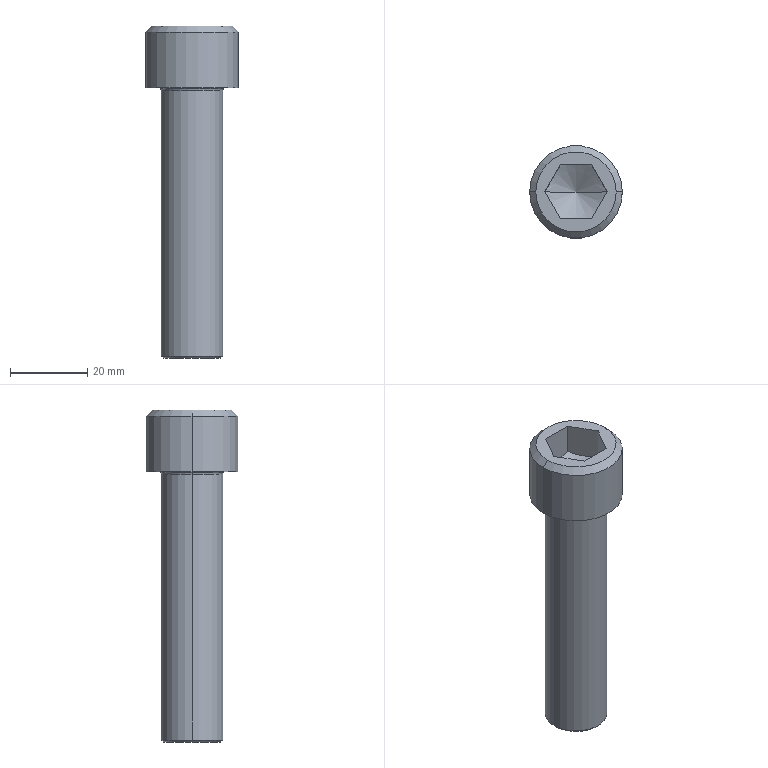Part | Creo | 1 solid | 23 faces | box 24 x 24 x 86 mm | volume 19550 mm3 | plane 9 | cone 6 | cylinder 4 | torus 4 | commonest cylinder face diameters 16 x2 24 x2
STEP:
#1=CARTESIAN_POINT('',(253.083,119.995,322.56));
#2=VERTEX_POINT('',#1);
#3=CARTESIAN_POINT('',(249.041,126.995,322.56));
#4=VERTEX_POINT('',#3);
#5=CARTESIAN_POINT('',(253.083,119.995,322.56));
#6=CARTESIAN_POINT('',(252.894,120.322,322.451));
#7=CARTESIAN_POINT('',(252.516,120.977,322.255));
#8=CARTESIAN_POINT('',(251.94,121.975,322.043));
#9=CARTESIAN_POINT('',(251.358,122.984,321.93));
#10=CARTESIAN_POINT('',(250.769,124.003,321.93));
#11=CARTESIAN_POINT('',(250.186,125.014,322.043));
#12=CARTESIAN_POINT('',(249.61,126.01,322.254));
#13=CARTESIAN_POINT('',(249.231,126.667,322.451));
#14=CARTESIAN_POINT('',(249.041,126.995,322.56));
#15=B_SPLINE_CURVE_WITH_KNOTS('',3,(#5,#6,#7,#8,#9,#10,#11,#12,#13,#14),.UNSPECIFIED.,.F.,.F.,(4,1,1,1,1,1,1,4),(0.,0.1429,0.2857,0.4286,0.5714,0.7143,0.8571,1.),.UNSPECIFIED.);
#16=EDGE_CURVE('',#2,#4,#15,.T.);
#17=ORIENTED_EDGE('',*,*,#16,.F.);
#18=CARTESIAN_POINT('',(245.,119.995,317.893));
#19=VERTEX_POINT('',#18);
#20=CARTESIAN_POINT('',(245.,119.995,317.893));
#21=DIRECTION('',(0.866,0.,0.5));
#22=VECTOR('',#21,9.333);
#23=LINE('',#20,#22);
#24=EDGE_CURVE('',#19,#2,#23,.T.);
#25=ORIENTED_EDGE('',*,*,#24,.F.);
#26=CARTESIAN_POINT('',(236.917,119.995,322.56));
#27=VERTEX_POINT('',#26);
#28=CARTESIAN_POINT('',(245.,119.995,317.893));
#29=DIRECTION('',(-0.866,0.,0.5));
#30=VECTOR('',#29,9.333);
#31=LINE('',#28,#30);
#32=EDGE_CURVE('',#19,#27,#31,.T.);
#33=ORIENTED_EDGE('',*,*,#32,.T.);
#34=CARTESIAN_POINT('',(240.959,126.995,322.56));
#35=VERTEX_POINT('',#34);
#36=CARTESIAN_POINT('',(240.959,126.995,322.56));
#37=CARTESIAN_POINT('',(240.77,126.669,322.451));
#38=CARTESIAN_POINT('',(240.391,126.013,322.255));
#39=CARTESIAN_POINT('',(239.816,125.016,322.043));
#40=CARTESIAN_POINT('',(239.233,124.007,321.93));
#41=CARTESIAN_POINT('',(238.644,122.987,321.93));
#42=CARTESIAN_POINT('',(238.061,121.977,322.043));
#43=CARTESIAN_POINT('',(237.486,120.981,322.254));
#44=CARTESIAN_POINT('',(237.106,120.323,322.451));
#45=CARTESIAN_POINT('',(236.917,119.995,322.56));
#46=B_SPLINE_CURVE_WITH_KNOTS('',3,(#36,#37,#38,#39,#40,#41,#42,#43,#44,#45),.UNSPECIFIED.,.F.,.F.,(4,1,1,1,1,1,1,4),(0.,0.1429,0.2857,0.4286,0.5714,0.7143,0.8571,1.),.UNSPECIFIED.);
#47=EDGE_CURVE('',#35,#27,#46,.T.);
#48=ORIENTED_EDGE('',*,*,#47,.F.);
#49=CARTESIAN_POINT('',(249.041,126.995,322.56));
#50=CARTESIAN_POINT('',(248.667,126.995,322.452));
#51=CARTESIAN_POINT('',(247.914,126.995,322.257));
#52=CARTESIAN_POINT('',(246.756,126.995,322.043));
#53=CARTESIAN_POINT('',(245.587,126.995,321.93));
#54=CARTESIAN_POINT('',(244.417,126.995,321.93));
#55=CARTESIAN_POINT('',(243.25,126.995,322.042));
#56=CARTESIAN_POINT('',(242.092,126.995,322.255));
#57=CARTESIAN_POINT('',(241.335,126.995,322.451));
#58=CARTESIAN_POINT('',(240.959,126.995,322.56));
#59=B_SPLINE_CURVE_WITH_KNOTS('',3,(#49,#50,#51,#52,#53,#54,#55,#56,#57,#58),.UNSPECIFIED.,.F.,.F.,(4,1,1,1,1,1,1,4),(0.,0.1429,0.2857,0.4286,0.5714,0.7143,0.8571,1.),.UNSPECIFIED.);
#60=EDGE_CURVE('',#4,#35,#59,.T.);
#61=ORIENTED_EDGE('',*,*,#60,.F.);
#62=EDGE_LOOP('',(#17,#25,#33,#48,#61));
#63=FACE_OUTER_BOUND('',#62,.F.);
#64=CARTESIAN_POINT('',(245.,119.995,320.273));
#65=DIRECTION('',(0.,0.,1.));
#66=DIRECTION('',(1.,0.,0.));
#67=AXIS2_PLACEMENT_3D('',#64,#65,#66);
#68=CONICAL_SURFACE('',#67,4.122,60.);
#69=ADVANCED_FACE('',(#63),#68,.F.);
#70=CARTESIAN_POINT('',(249.041,126.995,330.56));
#71=VERTEX_POINT('',#70);
#72=CARTESIAN_POINT('',(253.083,119.995,330.56));
#73=VERTEX_POINT('',#72);
#74=CARTESIAN_POINT('',(249.041,126.995,330.56));
#75=DIRECTION('',(0.5,-0.866,0.));
#76=VECTOR('',#75,8.083);
#77=LINE('',#74,#76);
#78=EDGE_CURVE('',#71,#73,#77,.T.);
#79=ORIENTED_EDGE('',*,*,#78,.T.);
#80=CARTESIAN_POINT('',(253.083,119.995,330.56));
#81=DIRECTION('',(0.,0.,-1.));
#82=VECTOR('',#81,8.);
#83=LINE('',#80,#82);
#84=EDGE_CURVE('',#73,#2,#83,.T.);
#85=ORIENTED_EDGE('',*,*,#84,.T.);
#86=ORIENTED_EDGE('',*,*,#16,.T.);
#87=CARTESIAN_POINT('',(249.041,126.995,330.56));
#88=DIRECTION('',(0.,0.,-1.));
#89=VECTOR('',#88,8.);
#90=LINE('',#87,#89);
#91=EDGE_CURVE('',#71,#4,#90,.T.);
#92=ORIENTED_EDGE('',*,*,#91,.F.);
#93=EDGE_LOOP('',(#79,#85,#86,#92));
#94=FACE_OUTER_BOUND('',#93,.F.);
#95=CARTESIAN_POINT('',(249.041,126.995,322.56));
#96=DIRECTION('',(-0.866,-0.5,0.));
#97=DIRECTION('',(0.5,-0.866,0.));
#98=AXIS2_PLACEMENT_3D('',#95,#96,#97);
#99=PLANE('',#98);
#100=ADVANCED_FACE('',(#94),#99,.T.);
#101=CARTESIAN_POINT('',(255.4,119.995,330.56));
#102=VERTEX_POINT('',#101);
#103=CARTESIAN_POINT('',(234.6,119.995,330.56));
#104=VERTEX_POINT('',#103);
#105=CARTESIAN_POINT('',(245.,119.995,330.56));
#106=DIRECTION('',(0.,0.,1.));
#107=DIRECTION('',(1.,0.,0.));
#108=AXIS2_PLACEMENT_3D('',#105,#106,#107);
#109=CIRCLE('',#108,10.4);
#110=EDGE_CURVE('',#102,#104,#109,.T.);
#111=ORIENTED_EDGE('',*,*,#110,.F.);
#112=CARTESIAN_POINT('',(245.,119.995,330.56));
#113=DIRECTION('',(0.,0.,1.));
#114=DIRECTION('',(-1.,0.,0.));
#115=AXIS2_PLACEMENT_3D('',#112,#113,#114);
#116=CIRCLE('',#115,10.4);
#117=EDGE_CURVE('',#104,#102,#116,.T.);
#118=ORIENTED_EDGE('',*,*,#117,.F.);
#119=EDGE_LOOP('',(#111,#118));
#120=FACE_OUTER_BOUND('',#119,.F.);
#121=CARTESIAN_POINT('',(249.041,112.995,330.56));
#122=VERTEX_POINT('',#121);
#123=CARTESIAN_POINT('',(253.083,119.995,330.56));
#124=DIRECTION('',(-0.5,-0.866,0.));
#125=VECTOR('',#124,8.083);
#126=LINE('',#123,#125);
#127=EDGE_CURVE('',#73,#122,#126,.T.);
#128=ORIENTED_EDGE('',*,*,#127,.F.);
#129=ORIENTED_EDGE('',*,*,#78,.F.);
#130=CARTESIAN_POINT('',(240.959,126.995,330.56));
#131=VERTEX_POINT('',#130);
#132=CARTESIAN_POINT('',(249.041,126.995,330.56));
#133=DIRECTION('',(-1.,0.,0.));
#134=VECTOR('',#133,8.083);
#135=LINE('',#132,#134);
#136=EDGE_CURVE('',#71,#131,#135,.T.);
#137=ORIENTED_EDGE('',*,*,#136,.T.);
#138=CARTESIAN_POINT('',(236.917,119.995,330.56));
#139=VERTEX_POINT('',#138);
#140=CARTESIAN_POINT('',(236.917,119.995,330.56));
#141=DIRECTION('',(0.5,0.866,0.));
#142=VECTOR('',#141,8.083);
#143=LINE('',#140,#142);
#144=EDGE_CURVE('',#139,#131,#143,.T.);
#145=ORIENTED_EDGE('',*,*,#144,.F.);
#146=CARTESIAN_POINT('',(240.959,112.995,330.56));
#147=VERTEX_POINT('',#146);
#148=CARTESIAN_POINT('',(240.959,112.995,330.56));
#149=DIRECTION('',(-0.5,0.866,0.));
#150=VECTOR('',#149,8.083);
#151=LINE('',#148,#150);
#152=EDGE_CURVE('',#147,#139,#151,.T.);
#153=ORIENTED_EDGE('',*,*,#152,.F.);
#154=CARTESIAN_POINT('',(240.959,112.995,330.56));
#155=DIRECTION('',(1.,0.,0.));
#156=VECTOR('',#155,8.083);
#157=LINE('',#154,#156);
#158=EDGE_CURVE('',#147,#122,#157,.T.);
#159=ORIENTED_EDGE('',*,*,#158,.T.);
#160=EDGE_LOOP('',(#128,#129,#137,#145,#153,#159));
#161=FACE_BOUND('',#160,.F.);
#162=CARTESIAN_POINT('',(245.,119.995,330.56));
#163=DIRECTION('',(0.,0.,1.));
#164=DIRECTION('',(1.,0.,0.));
#165=AXIS2_PLACEMENT_3D('',#162,#163,#164);
#166=PLANE('',#165);
#167=ADVANCED_FACE('',(#120,#161),#166,.T.);
#168=CARTESIAN_POINT('',(257.,119.995,328.96));
#169=VERTEX_POINT('',#168);
#170=CARTESIAN_POINT('',(233.,119.995,328.96));
#171=VERTEX_POINT('',#170);
#172=CARTESIAN_POINT('',(245.,119.995,328.96));
#173=DIRECTION('',(0.,0.,1.));
#174=DIRECTION('',(1.,0.,0.));
#175=AXIS2_PLACEMENT_3D('',#172,#173,#174);
#176=CIRCLE('',#175,12.);
#177=EDGE_CURVE('',#169,#171,#176,.T.);
#178=ORIENTED_EDGE('',*,*,#177,.F.);
#179=CARTESIAN_POINT('',(255.4,119.995,330.56));
#180=DIRECTION('',(0.7071,0.,-0.7071));
#181=VECTOR('',#180,2.263);
#182=LINE('',#179,#181);
#183=EDGE_CURVE('',#102,#169,#182,.T.);
#184=ORIENTED_EDGE('',*,*,#183,.F.);
#185=ORIENTED_EDGE('',*,*,#110,.T.);
#186=CARTESIAN_POINT('',(234.6,119.995,330.56));
#187=DIRECTION('',(-0.7071,0.,-0.7071));
#188=VECTOR('',#187,2.263);
#189=LINE('',#186,#188);
#190=EDGE_CURVE('',#104,#171,#189,.T.);
#191=ORIENTED_EDGE('',*,*,#190,.T.);
#192=EDGE_LOOP('',(#178,#184,#185,#191));
#193=FACE_OUTER_BOUND('',#192,.F.);
#194=CARTESIAN_POINT('',(245.,119.995,329.76));
#195=DIRECTION('',(0.,0.,-1.));
#196=DIRECTION('',(-1.,0.,0.));
#197=AXIS2_PLACEMENT_3D('',#194,#195,#196);
#198=CONICAL_SURFACE('',#197,11.2,45.);
#199=ADVANCED_FACE('',(#193),#198,.T.);
#200=ORIENTED_EDGE('',*,*,#177,.T.);
#201=CARTESIAN_POINT('',(233.,119.995,314.56));
#202=VERTEX_POINT('',#201);
#203=CARTESIAN_POINT('',(233.,119.995,314.56));
#204=DIRECTION('',(0.,0.,1.));
#205=VECTOR('',#204,14.4);
#206=LINE('',#203,#205);
#207=EDGE_CURVE('',#202,#171,#206,.T.);
#208=ORIENTED_EDGE('',*,*,#207,.F.);
#209=CARTESIAN_POINT('',(257.,119.995,314.56));
#210=VERTEX_POINT('',#209);
#211=CARTESIAN_POINT('',(245.,119.995,314.56));
#212=DIRECTION('',(0.,0.,-1.));
#213=DIRECTION('',(-1.,0.,0.));
#214=AXIS2_PLACEMENT_3D('',#211,#212,#213);
#215=CIRCLE('',#214,12.);
#216=EDGE_CURVE('',#202,#210,#215,.T.);
#217=ORIENTED_EDGE('',*,*,#216,.T.);
#218=CARTESIAN_POINT('',(257.,119.995,314.56));
#219=DIRECTION('',(0.,0.,1.));
#220=VECTOR('',#219,14.4);
#221=LINE('',#218,#220);
#222=EDGE_CURVE('',#210,#169,#221,.T.);
#223=ORIENTED_EDGE('',*,*,#222,.T.);
#224=EDGE_LOOP('',(#200,#208,#217,#223));
#225=FACE_OUTER_BOUND('',#224,.F.);
#226=CARTESIAN_POINT('',(245.,119.995,314.56));
#227=DIRECTION('',(0.,0.,1.));
#228=DIRECTION('',(1.,0.,0.));
#229=AXIS2_PLACEMENT_3D('',#226,#227,#228);
#230=CYLINDRICAL_SURFACE('',#229,12.);
#231=ADVANCED_FACE('',(#225),#230,.T.);
#232=CARTESIAN_POINT('',(245.,119.995,328.96));
#233=DIRECTION('',(0.,0.,1.));
#234=DIRECTION('',(-1.,0.,0.));
#235=AXIS2_PLACEMENT_3D('',#232,#233,#234);
#236=CIRCLE('',#235,12.);
#237=EDGE_CURVE('',#171,#169,#236,.T.);
#238=ORIENTED_EDGE('',*,*,#237,.T.);
#239=ORIENTED_EDGE('',*,*,#222,.F.);
#240=CARTESIAN_POINT('',(245.,119.995,314.56));
#241=DIRECTION('',(0.,0.,-1.));
#242=DIRECTION('',(1.,0.,0.));
#243=AXIS2_PLACEMENT_3D('',#240,#241,#242);
#244=CIRCLE('',#243,12.);
#245=EDGE_CURVE('',#210,#202,#244,.T.);
#246=ORIENTED_EDGE('',*,*,#245,.T.);
#247=ORIENTED_EDGE('',*,*,#207,.T.);
#248=EDGE_LOOP('',(#238,#239,#246,#247));
#249=FACE_OUTER_BOUND('',#248,.F.);
#250=CARTESIAN_POINT('',(245.,119.995,314.56));
#251=DIRECTION('',(0.,0.,1.));
#252=DIRECTION('',(1.,0.,0.));
#253=AXIS2_PLACEMENT_3D('',#250,#251,#252);
#254=CYLINDRICAL_SURFACE('',#253,12.);
#255=ADVANCED_FACE('',(#249),#254,.T.);
#256=ORIENTED_EDGE('',*,*,#237,.F.);
#257=ORIENTED_EDGE('',*,*,#190,.F.);
#258=ORIENTED_EDGE('',*,*,#117,.T.);
#259=ORIENTED_EDGE('',*,*,#183,.T.);
#260=EDGE_LOOP('',(#256,#257,#258,#259));
#261=FACE_OUTER_BOUND('',#260,.F.);
#262=CARTESIAN_POINT('',(245.,119.995,329.76));
#263=DIRECTION('',(0.,0.,-1.));
#264=DIRECTION('',(-1.,0.,0.));
#265=AXIS2_PLACEMENT_3D('',#262,#263,#264);
#266=CONICAL_SURFACE('',#265,11.2,45.);
#267=ADVANCED_FACE('',(#261),#266,.T.);
#268=ORIENTED_EDGE('',*,*,#245,.F.);
#269=ORIENTED_EDGE('',*,*,#216,.F.);
#270=EDGE_LOOP('',(#268,#269));
#271=FACE_OUTER_BOUND('',#270,.F.);
#272=CARTESIAN_POINT('',(253.6,119.995,314.56));
#273=VERTEX_POINT('',#272);
#274=CARTESIAN_POINT('',(236.4,119.995,314.56));
#275=VERTEX_POINT('',#274);
#276=CARTESIAN_POINT('',(245.,119.995,314.56));
#277=DIRECTION('',(0.,0.,1.));
#278=DIRECTION('',(1.,0.,0.));
#279=AXIS2_PLACEMENT_3D('',#276,#277,#278);
#280=CIRCLE('',#279,8.6);
#281=EDGE_CURVE('',#273,#275,#280,.T.);
#282=ORIENTED_EDGE('',*,*,#281,.F.);
#283=CARTESIAN_POINT('',(245.,119.995,314.56));
#284=DIRECTION('',(0.,0.,1.));
#285=DIRECTION('',(-1.,0.,0.));
#286=AXIS2_PLACEMENT_3D('',#283,#284,#285);
#287=CIRCLE('',#286,8.6);
#288=EDGE_CURVE('',#275,#273,#287,.T.);
#289=ORIENTED_EDGE('',*,*,#288,.F.);
#290=EDGE_LOOP('',(#282,#289));
#291=FACE_BOUND('',#290,.F.);
#292=CARTESIAN_POINT('',(245.,119.995,314.56));
#293=DIRECTION('',(0.,0.,1.));
#294=DIRECTION('',(1.,0.,0.));
#295=AXIS2_PLACEMENT_3D('',#292,#293,#294);
#296=PLANE('',#295);
#297=ADVANCED_FACE('',(#271,#291),#296,.F.);
#298=ORIENTED_EDGE('',*,*,#281,.T.);
#299=CARTESIAN_POINT('',(236.824,119.995,314.384));
#300=VERTEX_POINT('',#299);
#301=CARTESIAN_POINT('',(236.4,119.995,313.96));
#302=DIRECTION('',(0.,1.,0.));
#303=DIRECTION('',(0.,0.,1.));
#304=AXIS2_PLACEMENT_3D('',#301,#302,#303);
#305=CIRCLE('',#304,0.6);
#306=EDGE_CURVE('',#275,#300,#305,.T.);
#307=ORIENTED_EDGE('',*,*,#306,.T.);
#308=CARTESIAN_POINT('',(253.176,119.995,314.384));
#309=VERTEX_POINT('',#308);
#310=CARTESIAN_POINT('',(245.,119.995,314.384));
#311=DIRECTION('',(0.,0.,1.));
#312=DIRECTION('',(1.,0.,0.));
#313=AXIS2_PLACEMENT_3D('',#310,#311,#312);
#314=CIRCLE('',#313,8.176);
#315=EDGE_CURVE('',#309,#300,#314,.T.);
#316=ORIENTED_EDGE('',*,*,#315,.F.);
#317=CARTESIAN_POINT('',(253.6,119.995,313.96));
#318=DIRECTION('',(0.,-1.,0.));
#319=DIRECTION('',(0.,0.,1.));
#320=AXIS2_PLACEMENT_3D('',#317,#318,#319);
#321=CIRCLE('',#320,0.6);
#322=EDGE_CURVE('',#273,#309,#321,.T.);
#323=ORIENTED_EDGE('',*,*,#322,.F.);
#324=EDGE_LOOP('',(#298,#307,#316,#323));
#325=FACE_OUTER_BOUND('',#324,.F.);
#326=CARTESIAN_POINT('',(245.,119.995,313.96));
#327=DIRECTION('',(0.,0.,1.));
#328=DIRECTION('',(1.,0.,0.));
#329=AXIS2_PLACEMENT_3D('',#326,#327,#328);
#330=TOROIDAL_SURFACE('',#329,8.6,0.6);
#331=ADVANCED_FACE('',(#325),#330,.F.);
#332=ORIENTED_EDGE('',*,*,#288,.T.);
#333=ORIENTED_EDGE('',*,*,#322,.T.);
#334=CARTESIAN_POINT('',(245.,119.995,314.384));
#335=DIRECTION('',(0.,0.,1.));
#336=DIRECTION('',(-1.,0.,0.));
#337=AXIS2_PLACEMENT_3D('',#334,#335,#336);
#338=CIRCLE('',#337,8.176);
#339=EDGE_CURVE('',#300,#309,#338,.T.);
#340=ORIENTED_EDGE('',*,*,#339,.F.);
#341=ORIENTED_EDGE('',*,*,#306,.F.);
#342=EDGE_LOOP('',(#332,#333,#340,#341));
#343=FACE_OUTER_BOUND('',#342,.F.);
#344=CARTESIAN_POINT('',(245.,119.995,313.96));
#345=DIRECTION('',(0.,0.,1.));
#346=DIRECTION('',(1.,0.,0.));
#347=AXIS2_PLACEMENT_3D('',#344,#345,#346);
#348=TOROIDAL_SURFACE('',#347,8.6,0.6);
#349=ADVANCED_FACE('',(#343),#348,.F.);
#350=CARTESIAN_POINT('',(237.,119.995,313.96));
#351=VERTEX_POINT('',#350);
#352=CARTESIAN_POINT('',(253.,119.995,313.96));
#353=VERTEX_POINT('',#352);
#354=CARTESIAN_POINT('',(245.,119.995,313.96));
#355=DIRECTION('',(0.,0.,1.));
#356=DIRECTION('',(-1.,0.,0.));
#357=AXIS2_PLACEMENT_3D('',#354,#355,#356);
#358=CIRCLE('',#357,8.);
#359=EDGE_CURVE('',#351,#353,#358,.T.);
#360=ORIENTED_EDGE('',*,*,#359,.F.);
#361=CARTESIAN_POINT('',(236.4,119.995,313.96));
#362=DIRECTION('',(0.,1.,0.));
#363=DIRECTION('',(0.7071,0.,0.7071));
#364=AXIS2_PLACEMENT_3D('',#361,#362,#363);
#365=CIRCLE('',#364,0.6);
#366=EDGE_CURVE('',#300,#351,#365,.T.);
#367=ORIENTED_EDGE('',*,*,#366,.F.);
#368=ORIENTED_EDGE('',*,*,#339,.T.);
#369=CARTESIAN_POINT('',(253.6,119.995,313.96));
#370=DIRECTION('',(0.,-1.,0.));
#371=DIRECTION('',(-0.7071,0.,0.7071));
#372=AXIS2_PLACEMENT_3D('',#369,#370,#371);
#373=CIRCLE('',#372,0.6);
#374=EDGE_CURVE('',#309,#353,#373,.T.);
#375=ORIENTED_EDGE('',*,*,#374,.T.);
#376=EDGE_LOOP('',(#360,#367,#368,#375));
#377=FACE_OUTER_BOUND('',#376,.F.);
#378=CARTESIAN_POINT('',(245.,119.995,313.96));
#379=DIRECTION('',(0.,0.,1.));
#380=DIRECTION('',(1.,0.,0.));
#381=AXIS2_PLACEMENT_3D('',#378,#379,#380);
#382=TOROIDAL_SURFACE('',#381,8.6,0.6);
#383=ADVANCED_FACE('',(#377),#382,.F.);
#384=CARTESIAN_POINT('',(253.,119.995,245.06));
#385=VERTEX_POINT('',#384);
#386=CARTESIAN_POINT('',(237.,119.995,245.06));
#387=VERTEX_POINT('',#386);
#388=CARTESIAN_POINT('',(245.,119.995,245.06));
#389=DIRECTION('',(0.,0.,-1.));
#390=DIRECTION('',(1.,0.,0.));
#391=AXIS2_PLACEMENT_3D('',#388,#389,#390);
#392=CIRCLE('',#391,8.);
#393=EDGE_CURVE('',#385,#387,#392,.T.);
#394=ORIENTED_EDGE('',*,*,#393,.T.);
#395=CARTESIAN_POINT('',(237.,119.995,245.06));
#396=DIRECTION('',(0.,0.,1.));
#397=VECTOR('',#396,68.9);
#398=LINE('',#395,#397);
#399=EDGE_CURVE('',#387,#351,#398,.T.);
#400=ORIENTED_EDGE('',*,*,#399,.T.);
#401=ORIENTED_EDGE('',*,*,#359,.T.);
#402=CARTESIAN_POINT('',(253.,119.995,245.06));
#403=DIRECTION('',(0.,0.,1.));
#404=VECTOR('',#403,68.9);
#405=LINE('',#402,#404);
#406=EDGE_CURVE('',#385,#353,#405,.T.);
#407=ORIENTED_EDGE('',*,*,#406,.F.);
#408=EDGE_LOOP('',(#394,#400,#401,#407));
#409=FACE_OUTER_BOUND('',#408,.F.);
#410=CARTESIAN_POINT('',(245.,119.995,244.56));
#411=DIRECTION('',(0.,0.,1.));
#412=DIRECTION('',(1.,0.,0.));
#413=AXIS2_PLACEMENT_3D('',#410,#411,#412);
#414=CYLINDRICAL_SURFACE('',#413,8.);
#415=ADVANCED_FACE('',(#409),#414,.T.);
#416=CARTESIAN_POINT('',(252.5,119.995,244.56));
#417=VERTEX_POINT('',#416);
#418=CARTESIAN_POINT('',(237.5,119.995,244.56));
#419=VERTEX_POINT('',#418);
#420=CARTESIAN_POINT('',(245.,119.995,244.56));
#421=DIRECTION('',(0.,0.,-1.));
#422=DIRECTION('',(1.,0.,0.));
#423=AXIS2_PLACEMENT_3D('',#420,#421,#422);
#424=CIRCLE('',#423,7.5);
#425=EDGE_CURVE('',#417,#419,#424,.T.);
#426=ORIENTED_EDGE('',*,*,#425,.T.);
#427=CARTESIAN_POINT('',(237.5,119.995,244.56));
#428=DIRECTION('',(-0.7071,0.,0.7071));
#429=VECTOR('',#428,0.7071);
#430=LINE('',#427,#429);
#431=EDGE_CURVE('',#419,#387,#430,.T.);
#432=ORIENTED_EDGE('',*,*,#431,.T.);
#433=ORIENTED_EDGE('',*,*,#393,.F.);
#434=CARTESIAN_POINT('',(252.5,119.995,244.56));
#435=DIRECTION('',(0.7071,0.,0.7071));
#436=VECTOR('',#435,0.7071);
#437=LINE('',#434,#436);
#438=EDGE_CURVE('',#417,#385,#437,.T.);
#439=ORIENTED_EDGE('',*,*,#438,.F.);
#440=EDGE_LOOP('',(#426,#432,#433,#439));
#441=FACE_OUTER_BOUND('',#440,.F.);
#442=CARTESIAN_POINT('',(245.,119.995,244.81));
#443=DIRECTION('',(0.,0.,1.));
#444=DIRECTION('',(1.,0.,0.));
#445=AXIS2_PLACEMENT_3D('',#442,#443,#444);
#446=CONICAL_SURFACE('',#445,7.75,45.);
#447=ADVANCED_FACE('',(#441),#446,.T.);
#448=ORIENTED_EDGE('',*,*,#425,.F.);
#449=CARTESIAN_POINT('',(245.,119.995,244.56));
#450=DIRECTION('',(0.,0.,-1.));
#451=DIRECTION('',(-1.,0.,0.));
#452=AXIS2_PLACEMENT_3D('',#449,#450,#451);
#453=CIRCLE('',#452,7.5);
#454=EDGE_CURVE('',#419,#417,#453,.T.);
#455=ORIENTED_EDGE('',*,*,#454,.F.);
#456=EDGE_LOOP('',(#448,#455));
#457=FACE_OUTER_BOUND('',#456,.F.);
#458=CARTESIAN_POINT('',(245.,119.995,244.56));
#459=DIRECTION('',(0.,0.,1.));
#460=DIRECTION('',(1.,0.,0.));
#461=AXIS2_PLACEMENT_3D('',#458,#459,#460);
#462=PLANE('',#461);
#463=ADVANCED_FACE('',(#457),#462,.F.);
#464=ORIENTED_EDGE('',*,*,#454,.T.);
#465=ORIENTED_EDGE('',*,*,#438,.T.);
#466=CARTESIAN_POINT('',(245.,119.995,245.06));
#467=DIRECTION('',(0.,0.,-1.));
#468=DIRECTION('',(-1.,0.,0.));
#469=AXIS2_PLACEMENT_3D('',#466,#467,#468);
#470=CIRCLE('',#469,8.);
#471=EDGE_CURVE('',#387,#385,#470,.T.);
#472=ORIENTED_EDGE('',*,*,#471,.F.);
#473=ORIENTED_EDGE('',*,*,#431,.F.);
#474=EDGE_LOOP('',(#464,#465,#472,#473));
#475=FACE_OUTER_BOUND('',#474,.F.);
#476=CARTESIAN_POINT('',(245.,119.995,244.81));
#477=DIRECTION('',(0.,0.,1.));
#478=DIRECTION('',(1.,0.,0.));
#479=AXIS2_PLACEMENT_3D('',#476,#477,#478);
#480=CONICAL_SURFACE('',#479,7.75,45.);
#481=ADVANCED_FACE('',(#475),#480,.T.);
#482=ORIENTED_EDGE('',*,*,#471,.T.);
#483=ORIENTED_EDGE('',*,*,#406,.T.);
#484=CARTESIAN_POINT('',(245.,119.995,313.96));
#485=DIRECTION('',(0.,0.,1.));
#486=DIRECTION('',(1.,0.,0.));
#487=AXIS2_PLACEMENT_3D('',#484,#485,#486);
#488=CIRCLE('',#487,8.);
#489=EDGE_CURVE('',#353,#351,#488,.T.);
#490=ORIENTED_EDGE('',*,*,#489,.T.);
#491=ORIENTED_EDGE('',*,*,#399,.F.);
#492=EDGE_LOOP('',(#482,#483,#490,#491));
#493=FACE_OUTER_BOUND('',#492,.F.);
#494=CARTESIAN_POINT('',(245.,119.995,244.56));
#495=DIRECTION('',(0.,0.,1.));
#496=DIRECTION('',(1.,0.,0.));
#497=AXIS2_PLACEMENT_3D('',#494,#495,#496);
#498=CYLINDRICAL_SURFACE('',#497,8.);
#499=ADVANCED_FACE('',(#493),#498,.T.);
#500=ORIENTED_EDGE('',*,*,#489,.F.);
#501=ORIENTED_EDGE('',*,*,#374,.F.);
#502=ORIENTED_EDGE('',*,*,#315,.T.);
#503=ORIENTED_EDGE('',*,*,#366,.T.);
#504=EDGE_LOOP('',(#500,#501,#502,#503));
#505=FACE_OUTER_BOUND('',#504,.F.);
#506=CARTESIAN_POINT('',(245.,119.995,313.96));
#507=DIRECTION('',(0.,0.,1.));
#508=DIRECTION('',(1.,0.,0.));
#509=AXIS2_PLACEMENT_3D('',#506,#507,#508);
#510=TOROIDAL_SURFACE('',#509,8.6,0.6);
#511=ADVANCED_FACE('',(#505),#510,.F.);
#512=ORIENTED_EDGE('',*,*,#127,.T.);
#513=CARTESIAN_POINT('',(249.041,112.995,322.56));
#514=VERTEX_POINT('',#513);
#515=CARTESIAN_POINT('',(249.041,112.995,330.56));
#516=DIRECTION('',(0.,0.,-1.));
#517=VECTOR('',#516,8.);
#518=LINE('',#515,#517);
#519=EDGE_CURVE('',#122,#514,#518,.T.);
#520=ORIENTED_EDGE('',*,*,#519,.T.);
#521=CARTESIAN_POINT('',(249.041,112.995,322.56));
#522=CARTESIAN_POINT('',(249.23,113.322,322.451));
#523=CARTESIAN_POINT('',(249.609,113.977,322.255));
#524=CARTESIAN_POINT('',(250.184,114.975,322.043));
#525=CARTESIAN_POINT('',(250.767,115.984,321.93));
#526=CARTESIAN_POINT('',(251.356,117.003,321.93));
#527=CARTESIAN_POINT('',(251.939,118.014,322.043));
#528=CARTESIAN_POINT('',(252.514,119.01,322.254));
#529=CARTESIAN_POINT('',(252.894,119.667,322.451));
#530=CARTESIAN_POINT('',(253.083,119.995,322.56));
#531=B_SPLINE_CURVE_WITH_KNOTS('',3,(#521,#522,#523,#524,#525,#526,#527,#528,#529,#530),.UNSPECIFIED.,.F.,.F.,(4,1,1,1,1,1,1,4),(0.,0.1429,0.2857,0.4286,0.5714,0.7143,0.8571,1.),.UNSPECIFIED.);
#532=EDGE_CURVE('',#514,#2,#531,.T.);
#533=ORIENTED_EDGE('',*,*,#532,.T.);
#534=ORIENTED_EDGE('',*,*,#84,.F.);
#535=EDGE_LOOP('',(#512,#520,#533,#534));
#536=FACE_OUTER_BOUND('',#535,.F.);
#537=CARTESIAN_POINT('',(253.083,119.995,322.56));
#538=DIRECTION('',(-0.866,0.5,0.));
#539=DIRECTION('',(-0.5,-0.866,0.));
#540=AXIS2_PLACEMENT_3D('',#537,#538,#539);
#541=PLANE('',#540);
#542=ADVANCED_FACE('',(#536),#541,.T.);
#543=ORIENTED_EDGE('',*,*,#158,.F.);
#544=CARTESIAN_POINT('',(240.959,112.995,322.56));
#545=VERTEX_POINT('',#544);
#546=CARTESIAN_POINT('',(240.959,112.995,330.56));
#547=DIRECTION('',(0.,0.,-1.));
#548=VECTOR('',#547,8.);
#549=LINE('',#546,#548);
#550=EDGE_CURVE('',#147,#545,#549,.T.);
#551=ORIENTED_EDGE('',*,*,#550,.T.);
#552=CARTESIAN_POINT('',(240.959,112.995,322.56));
#553=CARTESIAN_POINT('',(241.335,112.995,322.451));
#554=CARTESIAN_POINT('',(242.092,112.995,322.255));
#555=CARTESIAN_POINT('',(243.25,112.995,322.042));
#556=CARTESIAN_POINT('',(244.417,112.995,321.93));
#557=CARTESIAN_POINT('',(245.587,112.995,321.93));
#558=CARTESIAN_POINT('',(246.756,112.995,322.043));
#559=CARTESIAN_POINT('',(247.914,112.995,322.257));
#560=CARTESIAN_POINT('',(248.667,112.995,322.452));
#561=CARTESIAN_POINT('',(249.041,112.995,322.56));
#562=B_SPLINE_CURVE_WITH_KNOTS('',3,(#552,#553,#554,#555,#556,#557,#558,#559,#560,#561),.UNSPECIFIED.,.F.,.F.,(4,1,1,1,1,1,1,4),(0.,0.1429,0.2857,0.4286,0.5714,0.7143,0.8571,1.),.UNSPECIFIED.);
#563=EDGE_CURVE('',#545,#514,#562,.T.);
#564=ORIENTED_EDGE('',*,*,#563,.T.);
#565=ORIENTED_EDGE('',*,*,#519,.F.);
#566=EDGE_LOOP('',(#543,#551,#564,#565));
#567=FACE_OUTER_BOUND('',#566,.F.);
#568=CARTESIAN_POINT('',(249.041,112.995,322.56));
#569=DIRECTION('',(0.,1.,0.));
#570=DIRECTION('',(0.,0.,1.));
#571=AXIS2_PLACEMENT_3D('',#568,#569,#570);
#572=PLANE('',#571);
#573=ADVANCED_FACE('',(#567),#572,.T.);
#574=ORIENTED_EDGE('',*,*,#152,.T.);
#575=CARTESIAN_POINT('',(236.917,119.995,330.56));
#576=DIRECTION('',(0.,0.,-1.));
#577=VECTOR('',#576,8.);
#578=LINE('',#575,#577);
#579=EDGE_CURVE('',#139,#27,#578,.T.);
#580=ORIENTED_EDGE('',*,*,#579,.T.);
#581=CARTESIAN_POINT('',(236.917,119.995,322.56));
#582=CARTESIAN_POINT('',(237.106,119.667,322.451));
#583=CARTESIAN_POINT('',(237.486,119.01,322.254));
#584=CARTESIAN_POINT('',(238.061,118.014,322.043));
#585=CARTESIAN_POINT('',(238.644,117.003,321.93));
#586=CARTESIAN_POINT('',(239.233,115.984,321.93));
#587=CARTESIAN_POINT('',(239.816,114.975,322.043));
#588=CARTESIAN_POINT('',(240.391,113.977,322.255));
#589=CARTESIAN_POINT('',(240.77,113.322,322.451));
#590=CARTESIAN_POINT('',(240.959,112.995,322.56));
#591=B_SPLINE_CURVE_WITH_KNOTS('',3,(#581,#582,#583,#584,#585,#586,#587,#588,#589,#590),.UNSPECIFIED.,.F.,.F.,(4,1,1,1,1,1,1,4),(0.,0.1429,0.2857,0.4286,0.5714,0.7143,0.8571,1.),.UNSPECIFIED.);
#592=EDGE_CURVE('',#27,#545,#591,.T.);
#593=ORIENTED_EDGE('',*,*,#592,.T.);
#594=ORIENTED_EDGE('',*,*,#550,.F.);
#595=EDGE_LOOP('',(#574,#580,#593,#594));
#596=FACE_OUTER_BOUND('',#595,.F.);
#597=CARTESIAN_POINT('',(240.959,112.995,322.56));
#598=DIRECTION('',(0.866,0.5,0.));
#599=DIRECTION('',(-0.5,0.866,0.));
#600=AXIS2_PLACEMENT_3D('',#597,#598,#599);
#601=PLANE('',#600);
#602=ADVANCED_FACE('',(#596),#601,.T.);
#603=ORIENTED_EDGE('',*,*,#144,.T.);
#604=CARTESIAN_POINT('',(240.959,126.995,330.56));
#605=DIRECTION('',(0.,0.,-1.));
#606=VECTOR('',#605,8.);
#607=LINE('',#604,#606);
#608=EDGE_CURVE('',#131,#35,#607,.T.);
#609=ORIENTED_EDGE('',*,*,#608,.T.);
#610=ORIENTED_EDGE('',*,*,#47,.T.);
#611=ORIENTED_EDGE('',*,*,#579,.F.);
#612=EDGE_LOOP('',(#603,#609,#610,#611));
#613=FACE_OUTER_BOUND('',#612,.F.);
#614=CARTESIAN_POINT('',(236.917,119.995,322.56));
#615=DIRECTION('',(0.866,-0.5,0.));
#616=DIRECTION('',(0.5,0.866,0.));
#617=AXIS2_PLACEMENT_3D('',#614,#615,#616);
#618=PLANE('',#617);
#619=ADVANCED_FACE('',(#613),#618,.T.);
#620=ORIENTED_EDGE('',*,*,#136,.F.);
#621=ORIENTED_EDGE('',*,*,#91,.T.);
#622=ORIENTED_EDGE('',*,*,#60,.T.);
#623=ORIENTED_EDGE('',*,*,#608,.F.);
#624=EDGE_LOOP('',(#620,#621,#622,#623));
#625=FACE_OUTER_BOUND('',#624,.F.);
#626=CARTESIAN_POINT('',(240.959,126.995,322.56));
#627=DIRECTION('',(0.,-1.,0.));
#628=DIRECTION('',(0.,0.,-1.));
#629=AXIS2_PLACEMENT_3D('',#626,#627,#628);
#630=PLANE('',#629);
#631=ADVANCED_FACE('',(#625),#630,.T.);
#632=ORIENTED_EDGE('',*,*,#592,.F.);
#633=ORIENTED_EDGE('',*,*,#32,.F.);
#634=ORIENTED_EDGE('',*,*,#24,.T.);
#635=ORIENTED_EDGE('',*,*,#532,.F.);
#636=ORIENTED_EDGE('',*,*,#563,.F.);
#637=EDGE_LOOP('',(#632,#633,#634,#635,#636));
#638=FACE_OUTER_BOUND('',#637,.F.);
#639=CARTESIAN_POINT('',(245.,119.995,320.273));
#640=DIRECTION('',(0.,0.,1.));
#641=DIRECTION('',(1.,0.,0.));
#642=AXIS2_PLACEMENT_3D('',#639,#640,#641);
#643=CONICAL_SURFACE('',#642,4.122,60.);
#644=ADVANCED_FACE('',(#638),#643,.F.);
#645=CLOSED_SHELL('',(#69,#100,#167,#199,#231,#255,#267,#297,#331,#349,#383,#415,#447,#463,#481,#499,#511,#542,#573,#602,#619,#631,#644));
#646=MANIFOLD_SOLID_BREP('',#645);
#647=(LENGTH_UNIT()NAMED_UNIT(*)SI_UNIT(.MILLI.,.METRE.));
#648=UNCERTAINTY_MEASURE_WITH_UNIT(LENGTH_MEASURE(0.009245),#647,'','');
#649=(NAMED_UNIT(*)PLANE_ANGLE_UNIT()SI_UNIT($,.RADIAN.));
#650=PLANE_ANGLE_MEASURE_WITH_UNIT(PLANE_ANGLE_MEASURE(0.01745),#649);
#651=(CONVERSION_BASED_UNIT('DEGREE',#650)NAMED_UNIT(*)PLANE_ANGLE_UNIT());
#652=(NAMED_UNIT(*)SI_UNIT($,.STERADIAN.)SOLID_ANGLE_UNIT());
#653=(GEOMETRIC_REPRESENTATION_CONTEXT(3)GLOBAL_UNCERTAINTY_ASSIGNED_CONTEXT((#648))GLOBAL_UNIT_ASSIGNED_CONTEXT((#647,#651,#652))REPRESENTATION_CONTEXT('',''));
#654=ADVANCED_BREP_SHAPE_REPRESENTATION('',(#646),#653);